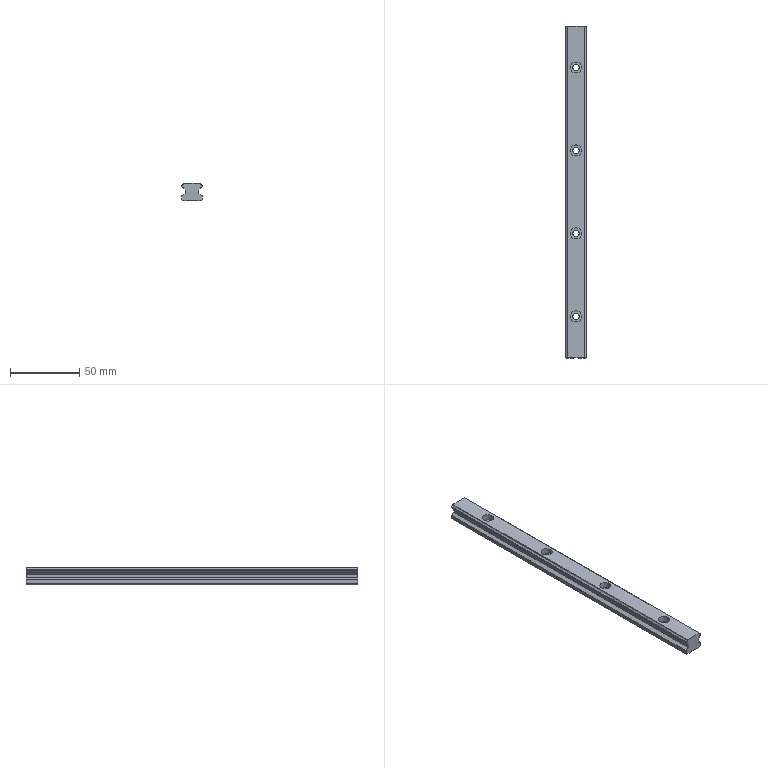Part | STEP file | linear guide EGH15CA-240-30-30_L=560 | 1 solid | 62 faces | box 15 x 240 x 12.5 mm | volume 36704 mm3 | plane 42 | cylinder 20 | commonest cylinder face diameters 4.5 x8 8 x8 3.1 x4